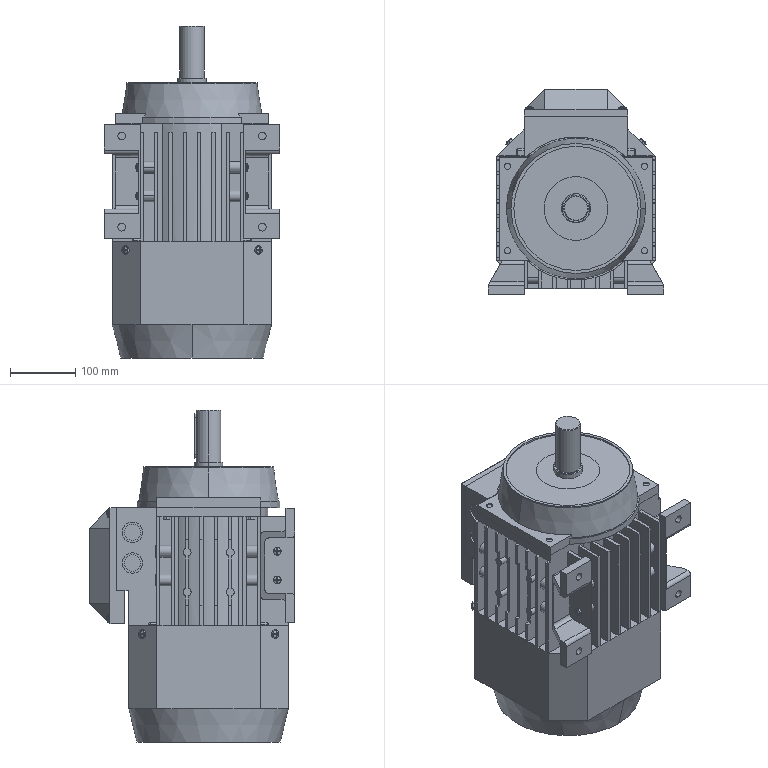Part | STEP file | IM B3 H63-132 variable-frequency motor [YVF2-132S2-4-B3]_YVF2-132S2-4-B3 | 1 solid | 1297 faces | box 270 x 315 x 510 mm | volume 20221478 mm3 | plane 1055 | cylinder 182 | torus 32 | sphere 20 | cone 8 | commonest cylinder face diameters 12 x32 183.75 x29 9.8 x24 12.25 x24 18 x18 3.92 x12